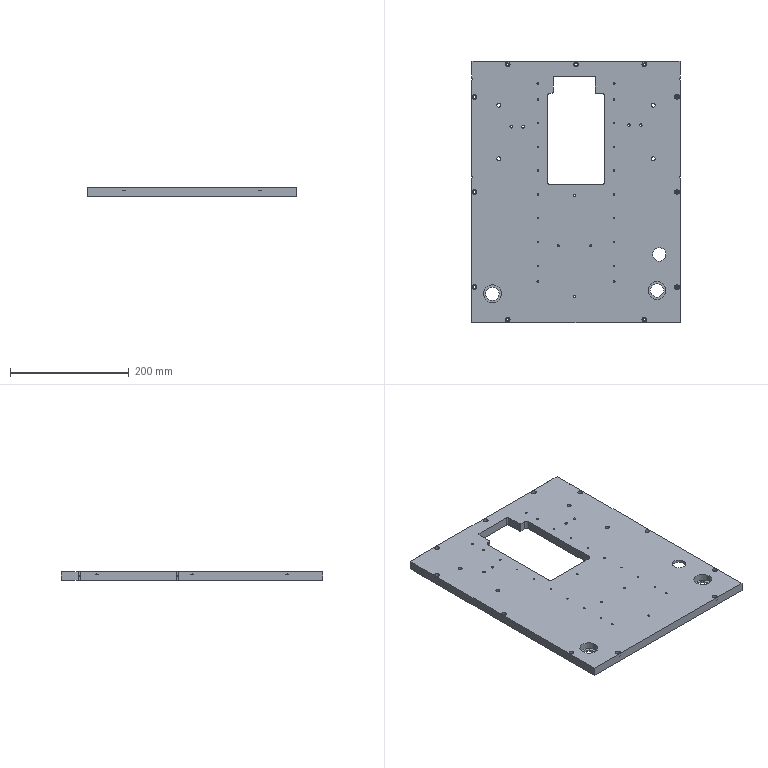Part | SolidWorks | features BaseBody 1 | 1 solid | 216 faces | box 350.001 x 440 x 15 mm | volume 1979972 mm3 | cylinder 168 | plane 48 | commonest cylinder face diameters 3.3 x34 2.5 x32 4.2 x30 8 x22 10 x20 6.6 x8